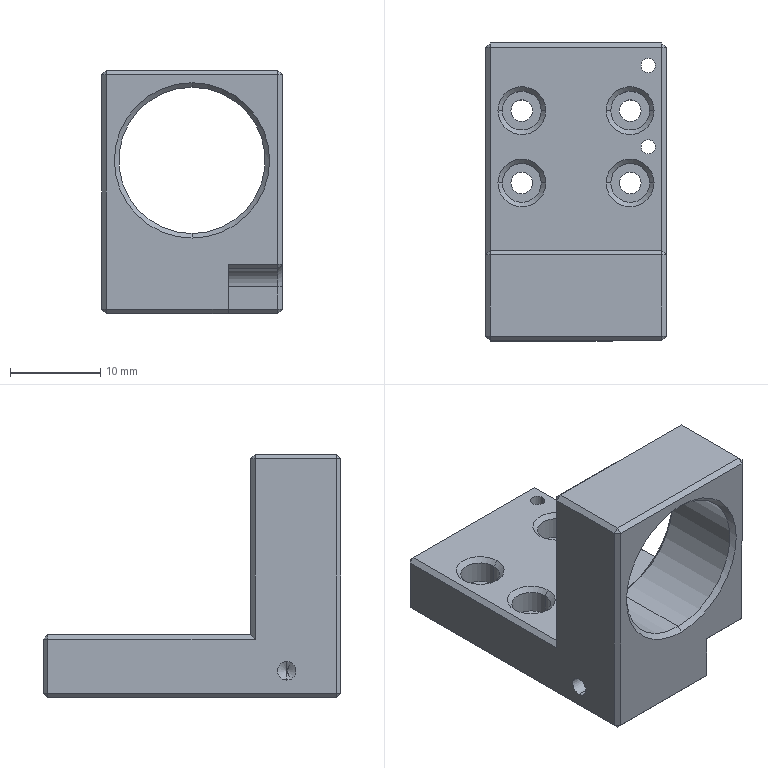Part | SolidWorks | features HoleWzd 5, ICE 2, Chamfer 1, Extrusion 1, Fillet 1 | 1 solid | 127 faces | box 20 x 33 x 27 mm | volume 5778 mm3 | plane 47 | cone 43 | cylinder 37 | commonest cylinder face diameters 2.05 x10 1.6 x8 2.4 x8 4.3 x8 16.2 x2 4 x1